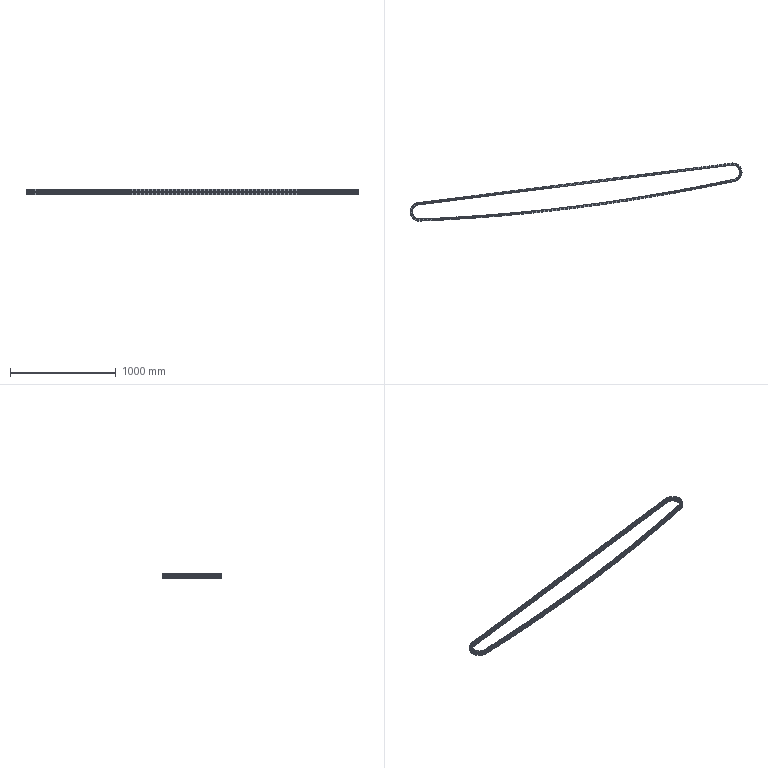Part | NX | features BREP 845 | 845 solids | 14047 faces | volume 2025822 mm3 | cylinder 7625 | plane 5070 | cone 1352 | commonest cylinder face diameters 5.96 x2704 18.08 x1873 5.5 x1352 83.184 x1020 11.91 x676